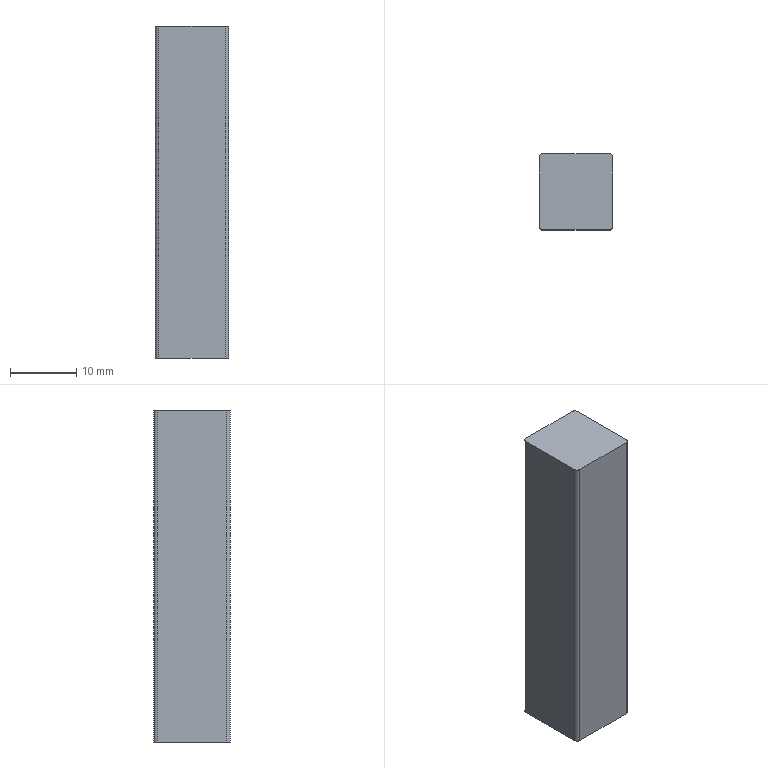Part | NX | features BREP 1 | 1 solid | 10 faces | box 11.003 x 11.506 x 50 mm | volume 6319 mm3 | plane 6 | cylinder 4 | commonest cylinder face diameters 1 x4
STEP:
#1=CARTESIAN_POINT('',(-5.002,5.753,-40.6));
#2=VERTEX_POINT('',#1);
#3=CARTESIAN_POINT('',(-5.502,5.253,-40.6));
#4=VERTEX_POINT('',#3);
#5=CARTESIAN_POINT('',(-5.002,5.253,-40.6));
#6=DIRECTION('',(0.,0.,1.));
#7=DIRECTION('',(1.,0.,0.));
#8=AXIS2_PLACEMENT_3D('',#5,#6,#7);
#9=CIRCLE('',#8,0.5);
#10=EDGE_CURVE('',#2,#4,#9,.T.);
#11=ORIENTED_EDGE('',*,*,#10,.F.);
#12=CARTESIAN_POINT('',(-5.002,5.753,-90.6));
#13=VERTEX_POINT('',#12);
#14=CARTESIAN_POINT('',(-5.002,5.753,-90.6));
#15=DIRECTION('',(0.,0.,1.));
#16=VECTOR('',#15,1000.);
#17=LINE('',#14,#16);
#18=EDGE_CURVE('',#13,#2,#17,.T.);
#19=ORIENTED_EDGE('',*,*,#18,.F.);
#20=CARTESIAN_POINT('',(-5.502,5.253,-90.6));
#21=VERTEX_POINT('',#20);
#22=CARTESIAN_POINT('',(-5.002,5.253,-90.6));
#23=DIRECTION('',(0.,0.,1.));
#24=DIRECTION('',(1.,0.,0.));
#25=AXIS2_PLACEMENT_3D('',#22,#23,#24);
#26=CIRCLE('',#25,0.5);
#27=EDGE_CURVE('',#13,#21,#26,.T.);
#28=ORIENTED_EDGE('',*,*,#27,.T.);
#29=CARTESIAN_POINT('',(-5.502,5.253,-90.6));
#30=DIRECTION('',(0.,0.,1.));
#31=VECTOR('',#30,1000.);
#32=LINE('',#29,#31);
#33=EDGE_CURVE('',#21,#4,#32,.T.);
#34=ORIENTED_EDGE('',*,*,#33,.T.);
#35=EDGE_LOOP('',(#11,#19,#28,#34));
#36=FACE_BOUND('',#35,.T.);
#37=CARTESIAN_POINT('',(-5.002,5.253,-90.6));
#38=DIRECTION('',(0.,0.,1.));
#39=DIRECTION('',(-1.,0.,0.));
#40=AXIS2_PLACEMENT_3D('',#37,#38,#39);
#41=CYLINDRICAL_SURFACE('',#40,0.5);
#42=ADVANCED_FACE('',(#36),#41,.T.);
#43=CARTESIAN_POINT('',(-5.502,-5.253,-40.6));
#44=VERTEX_POINT('',#43);
#45=CARTESIAN_POINT('',(-5.502,-5.253,-40.6));
#46=DIRECTION('',(0.,1.,0.));
#47=VECTOR('',#46,1000.);
#48=LINE('',#45,#47);
#49=EDGE_CURVE('',#44,#4,#48,.T.);
#50=ORIENTED_EDGE('',*,*,#49,.T.);
#51=ORIENTED_EDGE('',*,*,#33,.F.);
#52=CARTESIAN_POINT('',(-5.502,-5.253,-90.6));
#53=VERTEX_POINT('',#52);
#54=CARTESIAN_POINT('',(-5.502,-5.253,-90.6));
#55=DIRECTION('',(0.,1.,0.));
#56=VECTOR('',#55,1000.);
#57=LINE('',#54,#56);
#58=EDGE_CURVE('',#53,#21,#57,.T.);
#59=ORIENTED_EDGE('',*,*,#58,.F.);
#60=CARTESIAN_POINT('',(-5.502,-5.253,-90.6));
#61=DIRECTION('',(0.,0.,1.));
#62=VECTOR('',#61,1000.);
#63=LINE('',#60,#62);
#64=EDGE_CURVE('',#53,#44,#63,.T.);
#65=ORIENTED_EDGE('',*,*,#64,.T.);
#66=EDGE_LOOP('',(#50,#51,#59,#65));
#67=FACE_BOUND('',#66,.T.);
#68=CARTESIAN_POINT('',(-5.502,-5.253,-90.6));
#69=DIRECTION('',(1.,0.,0.));
#70=DIRECTION('',(0.,-1.,0.));
#71=AXIS2_PLACEMENT_3D('',#68,#69,#70);
#72=PLANE('',#71);
#73=ADVANCED_FACE('',(#67),#72,.F.);
#74=CARTESIAN_POINT('',(-5.002,-5.753,-40.6));
#75=VERTEX_POINT('',#74);
#76=CARTESIAN_POINT('',(-5.002,-5.253,-40.6));
#77=DIRECTION('',(0.,0.,1.));
#78=DIRECTION('',(1.,0.,0.));
#79=AXIS2_PLACEMENT_3D('',#76,#77,#78);
#80=CIRCLE('',#79,0.5);
#81=EDGE_CURVE('',#44,#75,#80,.T.);
#82=ORIENTED_EDGE('',*,*,#81,.F.);
#83=ORIENTED_EDGE('',*,*,#64,.F.);
#84=CARTESIAN_POINT('',(-5.002,-5.753,-90.6));
#85=VERTEX_POINT('',#84);
#86=CARTESIAN_POINT('',(-5.002,-5.253,-90.6));
#87=DIRECTION('',(0.,0.,1.));
#88=DIRECTION('',(1.,0.,0.));
#89=AXIS2_PLACEMENT_3D('',#86,#87,#88);
#90=CIRCLE('',#89,0.5);
#91=EDGE_CURVE('',#53,#85,#90,.T.);
#92=ORIENTED_EDGE('',*,*,#91,.T.);
#93=CARTESIAN_POINT('',(-5.002,-5.753,-90.6));
#94=DIRECTION('',(0.,0.,1.));
#95=VECTOR('',#94,1000.);
#96=LINE('',#93,#95);
#97=EDGE_CURVE('',#85,#75,#96,.T.);
#98=ORIENTED_EDGE('',*,*,#97,.T.);
#99=EDGE_LOOP('',(#82,#83,#92,#98));
#100=FACE_BOUND('',#99,.T.);
#101=CARTESIAN_POINT('',(-5.002,-5.253,-90.6));
#102=DIRECTION('',(0.,0.,1.));
#103=DIRECTION('',(-1.,0.,0.));
#104=AXIS2_PLACEMENT_3D('',#101,#102,#103);
#105=CYLINDRICAL_SURFACE('',#104,0.5);
#106=ADVANCED_FACE('',(#100),#105,.T.);
#107=CARTESIAN_POINT('',(5.002,-5.753,-40.6));
#108=VERTEX_POINT('',#107);
#109=CARTESIAN_POINT('',(5.002,-5.753,-40.6));
#110=DIRECTION('',(-1.,0.,0.));
#111=VECTOR('',#110,1000.);
#112=LINE('',#109,#111);
#113=EDGE_CURVE('',#108,#75,#112,.T.);
#114=ORIENTED_EDGE('',*,*,#113,.T.);
#115=ORIENTED_EDGE('',*,*,#97,.F.);
#116=CARTESIAN_POINT('',(5.002,-5.753,-90.6));
#117=VERTEX_POINT('',#116);
#118=CARTESIAN_POINT('',(5.002,-5.753,-90.6));
#119=DIRECTION('',(-1.,0.,0.));
#120=VECTOR('',#119,1000.);
#121=LINE('',#118,#120);
#122=EDGE_CURVE('',#117,#85,#121,.T.);
#123=ORIENTED_EDGE('',*,*,#122,.F.);
#124=CARTESIAN_POINT('',(5.002,-5.753,-90.6));
#125=DIRECTION('',(0.,0.,1.));
#126=VECTOR('',#125,1000.);
#127=LINE('',#124,#126);
#128=EDGE_CURVE('',#117,#108,#127,.T.);
#129=ORIENTED_EDGE('',*,*,#128,.T.);
#130=EDGE_LOOP('',(#114,#115,#123,#129));
#131=FACE_BOUND('',#130,.T.);
#132=CARTESIAN_POINT('',(5.002,-5.753,-90.6));
#133=DIRECTION('',(0.,1.,0.));
#134=DIRECTION('',(1.,0.,0.));
#135=AXIS2_PLACEMENT_3D('',#132,#133,#134);
#136=PLANE('',#135);
#137=ADVANCED_FACE('',(#131),#136,.F.);
#138=CARTESIAN_POINT('',(5.502,-5.253,-40.6));
#139=VERTEX_POINT('',#138);
#140=CARTESIAN_POINT('',(5.002,-5.253,-40.6));
#141=DIRECTION('',(0.,0.,1.));
#142=DIRECTION('',(1.,0.,0.));
#143=AXIS2_PLACEMENT_3D('',#140,#141,#142);
#144=CIRCLE('',#143,0.5);
#145=EDGE_CURVE('',#108,#139,#144,.T.);
#146=ORIENTED_EDGE('',*,*,#145,.F.);
#147=ORIENTED_EDGE('',*,*,#128,.F.);
#148=CARTESIAN_POINT('',(5.502,-5.253,-90.6));
#149=VERTEX_POINT('',#148);
#150=CARTESIAN_POINT('',(5.002,-5.253,-90.6));
#151=DIRECTION('',(0.,0.,1.));
#152=DIRECTION('',(1.,0.,0.));
#153=AXIS2_PLACEMENT_3D('',#150,#151,#152);
#154=CIRCLE('',#153,0.5);
#155=EDGE_CURVE('',#117,#149,#154,.T.);
#156=ORIENTED_EDGE('',*,*,#155,.T.);
#157=CARTESIAN_POINT('',(5.502,-5.253,-90.6));
#158=DIRECTION('',(0.,0.,1.));
#159=VECTOR('',#158,1000.);
#160=LINE('',#157,#159);
#161=EDGE_CURVE('',#149,#139,#160,.T.);
#162=ORIENTED_EDGE('',*,*,#161,.T.);
#163=EDGE_LOOP('',(#146,#147,#156,#162));
#164=FACE_BOUND('',#163,.T.);
#165=CARTESIAN_POINT('',(5.002,-5.253,-90.6));
#166=DIRECTION('',(0.,0.,1.));
#167=DIRECTION('',(-1.,0.,0.));
#168=AXIS2_PLACEMENT_3D('',#165,#166,#167);
#169=CYLINDRICAL_SURFACE('',#168,0.5);
#170=ADVANCED_FACE('',(#164),#169,.T.);
#171=CARTESIAN_POINT('',(5.502,5.253,-40.6));
#172=VERTEX_POINT('',#171);
#173=CARTESIAN_POINT('',(5.502,5.253,-40.6));
#174=DIRECTION('',(0.,-1.,0.));
#175=VECTOR('',#174,1000.);
#176=LINE('',#173,#175);
#177=EDGE_CURVE('',#172,#139,#176,.T.);
#178=ORIENTED_EDGE('',*,*,#177,.T.);
#179=ORIENTED_EDGE('',*,*,#161,.F.);
#180=CARTESIAN_POINT('',(5.502,5.253,-90.6));
#181=VERTEX_POINT('',#180);
#182=CARTESIAN_POINT('',(5.502,5.253,-90.6));
#183=DIRECTION('',(0.,-1.,0.));
#184=VECTOR('',#183,1000.);
#185=LINE('',#182,#184);
#186=EDGE_CURVE('',#181,#149,#185,.T.);
#187=ORIENTED_EDGE('',*,*,#186,.F.);
#188=CARTESIAN_POINT('',(5.502,5.253,-90.6));
#189=DIRECTION('',(0.,0.,1.));
#190=VECTOR('',#189,1000.);
#191=LINE('',#188,#190);
#192=EDGE_CURVE('',#181,#172,#191,.T.);
#193=ORIENTED_EDGE('',*,*,#192,.T.);
#194=EDGE_LOOP('',(#178,#179,#187,#193));
#195=FACE_BOUND('',#194,.T.);
#196=CARTESIAN_POINT('',(5.502,5.253,-90.6));
#197=DIRECTION('',(-1.,0.,0.));
#198=DIRECTION('',(0.,0.,-1.));
#199=AXIS2_PLACEMENT_3D('',#196,#197,#198);
#200=PLANE('',#199);
#201=ADVANCED_FACE('',(#195),#200,.F.);
#202=CARTESIAN_POINT('',(5.002,5.753,-40.6));
#203=VERTEX_POINT('',#202);
#204=CARTESIAN_POINT('',(5.002,5.253,-40.6));
#205=DIRECTION('',(0.,0.,1.));
#206=DIRECTION('',(1.,0.,0.));
#207=AXIS2_PLACEMENT_3D('',#204,#205,#206);
#208=CIRCLE('',#207,0.5);
#209=EDGE_CURVE('',#172,#203,#208,.T.);
#210=ORIENTED_EDGE('',*,*,#209,.F.);
#211=ORIENTED_EDGE('',*,*,#192,.F.);
#212=CARTESIAN_POINT('',(5.002,5.753,-90.6));
#213=VERTEX_POINT('',#212);
#214=CARTESIAN_POINT('',(5.002,5.253,-90.6));
#215=DIRECTION('',(0.,0.,1.));
#216=DIRECTION('',(1.,0.,0.));
#217=AXIS2_PLACEMENT_3D('',#214,#215,#216);
#218=CIRCLE('',#217,0.5);
#219=EDGE_CURVE('',#181,#213,#218,.T.);
#220=ORIENTED_EDGE('',*,*,#219,.T.);
#221=CARTESIAN_POINT('',(5.002,5.753,-90.6));
#222=DIRECTION('',(0.,0.,1.));
#223=VECTOR('',#222,1000.);
#224=LINE('',#221,#223);
#225=EDGE_CURVE('',#213,#203,#224,.T.);
#226=ORIENTED_EDGE('',*,*,#225,.T.);
#227=EDGE_LOOP('',(#210,#211,#220,#226));
#228=FACE_BOUND('',#227,.T.);
#229=CARTESIAN_POINT('',(5.002,5.253,-90.6));
#230=DIRECTION('',(0.,0.,1.));
#231=DIRECTION('',(-1.,0.,0.));
#232=AXIS2_PLACEMENT_3D('',#229,#230,#231);
#233=CYLINDRICAL_SURFACE('',#232,0.5);
#234=ADVANCED_FACE('',(#228),#233,.T.);
#235=CARTESIAN_POINT('',(-5.002,5.753,-40.6));
#236=DIRECTION('',(1.,0.,0.));
#237=VECTOR('',#236,1000.);
#238=LINE('',#235,#237);
#239=EDGE_CURVE('',#2,#203,#238,.T.);
#240=ORIENTED_EDGE('',*,*,#239,.T.);
#241=ORIENTED_EDGE('',*,*,#225,.F.);
#242=CARTESIAN_POINT('',(-5.002,5.753,-90.6));
#243=DIRECTION('',(1.,0.,0.));
#244=VECTOR('',#243,1000.);
#245=LINE('',#242,#244);
#246=EDGE_CURVE('',#13,#213,#245,.T.);
#247=ORIENTED_EDGE('',*,*,#246,.F.);
#248=ORIENTED_EDGE('',*,*,#18,.T.);
#249=EDGE_LOOP('',(#240,#241,#247,#248));
#250=FACE_BOUND('',#249,.T.);
#251=CARTESIAN_POINT('',(-5.002,5.753,-90.6));
#252=DIRECTION('',(0.,-1.,0.));
#253=DIRECTION('',(0.,0.,1.));
#254=AXIS2_PLACEMENT_3D('',#251,#252,#253);
#255=PLANE('',#254);
#256=ADVANCED_FACE('',(#250),#255,.F.);
#257=ORIENTED_EDGE('',*,*,#27,.F.);
#258=ORIENTED_EDGE('',*,*,#246,.T.);
#259=ORIENTED_EDGE('',*,*,#219,.F.);
#260=ORIENTED_EDGE('',*,*,#186,.T.);
#261=ORIENTED_EDGE('',*,*,#155,.F.);
#262=ORIENTED_EDGE('',*,*,#122,.T.);
#263=ORIENTED_EDGE('',*,*,#91,.F.);
#264=ORIENTED_EDGE('',*,*,#58,.T.);
#265=EDGE_LOOP('',(#257,#258,#259,#260,#261,#262,#263,#264));
#266=FACE_BOUND('',#265,.T.);
#267=CARTESIAN_POINT('',(-5.002,5.253,-90.6));
#268=DIRECTION('',(0.,0.,1.));
#269=DIRECTION('',(-1.,0.,0.));
#270=AXIS2_PLACEMENT_3D('',#267,#268,#269);
#271=PLANE('',#270);
#272=ADVANCED_FACE('',(#266),#271,.F.);
#273=ORIENTED_EDGE('',*,*,#10,.T.);
#274=ORIENTED_EDGE('',*,*,#49,.F.);
#275=ORIENTED_EDGE('',*,*,#81,.T.);
#276=ORIENTED_EDGE('',*,*,#113,.F.);
#277=ORIENTED_EDGE('',*,*,#145,.T.);
#278=ORIENTED_EDGE('',*,*,#177,.F.);
#279=ORIENTED_EDGE('',*,*,#209,.T.);
#280=ORIENTED_EDGE('',*,*,#239,.F.);
#281=EDGE_LOOP('',(#273,#274,#275,#276,#277,#278,#279,#280));
#282=FACE_BOUND('',#281,.T.);
#283=CARTESIAN_POINT('',(-5.002,5.253,-40.6));
#284=DIRECTION('',(0.,0.,1.));
#285=DIRECTION('',(-1.,0.,0.));
#286=AXIS2_PLACEMENT_3D('',#283,#284,#285);
#287=PLANE('',#286);
#288=ADVANCED_FACE('',(#282),#287,.T.);
#289=CLOSED_SHELL('',(#42,#73,#106,#137,#170,#201,#234,#256,#272,#288));
#290=MANIFOLD_SOLID_BREP('',#289);
#291=(LENGTH_UNIT()NAMED_UNIT(*)SI_UNIT(.MILLI.,.METRE.));
#292=UNCERTAINTY_MEASURE_WITH_UNIT(LENGTH_MEASURE(0.00001),#291,'','');
#293=(NAMED_UNIT(*)PLANE_ANGLE_UNIT()SI_UNIT($,.RADIAN.));
#294=(NAMED_UNIT(*)SI_UNIT($,.STERADIAN.)SOLID_ANGLE_UNIT());
#295=(GEOMETRIC_REPRESENTATION_CONTEXT(3)GLOBAL_UNCERTAINTY_ASSIGNED_CONTEXT((#292))GLOBAL_UNIT_ASSIGNED_CONTEXT((#291,#293,#294))REPRESENTATION_CONTEXT('',''));
#296=ADVANCED_BREP_SHAPE_REPRESENTATION('',(#290),#295);